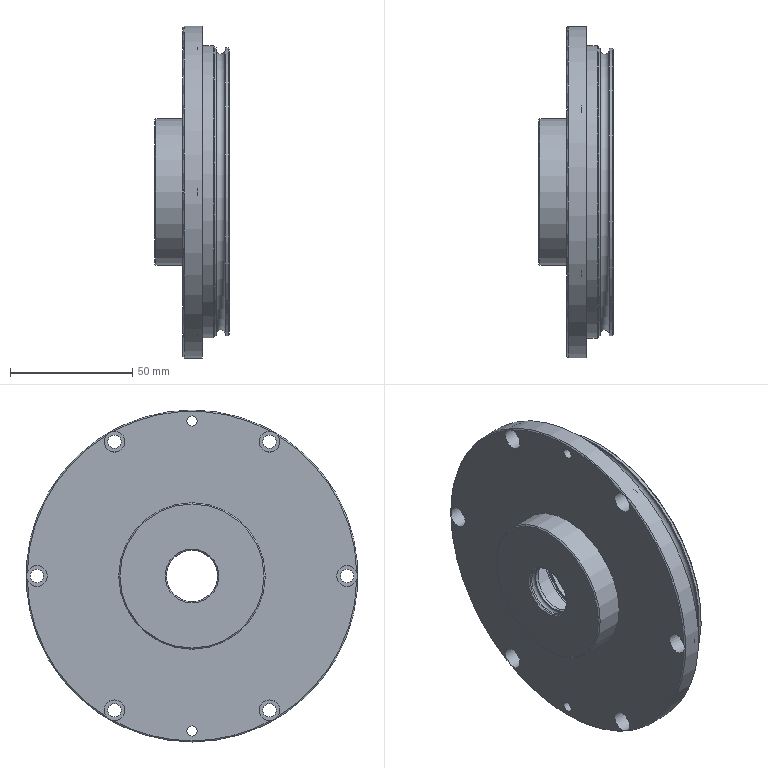Part | NX | features BREP 1 | 1 solid | 56 faces | box 30.5 x 136 x 136 mm | volume 150604 mm3 | cylinder 27 | plane 21 | cone 6 | torus 2 | commonest cylinder face diameters 5.5 x6 8.5 x6 4.2 x2 21 x2 47 x2 60 x2
STEP:
#1=CARTESIAN_POINT('',(13.3,0.,58.3));
#2=VERTEX_POINT('',#1);
#3=CARTESIAN_POINT('',(13.3,0.,0.));
#4=DIRECTION('',(-1.,0.,0.));
#5=DIRECTION('',(0.,0.,1.));
#6=AXIS2_PLACEMENT_3D('',#3,#4,#5);
#7=CIRCLE('',#6,58.3);
#8=EDGE_CURVE('',#2,#2,#7,.T.);
#9=ORIENTED_EDGE('',*,*,#8,.T.);
#10=EDGE_LOOP('',(#9));
#11=FACE_BOUND('',#10,.T.);
#12=CARTESIAN_POINT('',(9.7,0.,58.3));
#13=VERTEX_POINT('',#12);
#14=CARTESIAN_POINT('',(9.7,0.,0.));
#15=DIRECTION('',(-1.,0.,0.));
#16=DIRECTION('',(0.,0.,1.));
#17=AXIS2_PLACEMENT_3D('',#14,#15,#16);
#18=CIRCLE('',#17,58.3);
#19=EDGE_CURVE('',#13,#13,#18,.T.);
#20=ORIENTED_EDGE('',*,*,#19,.F.);
#21=EDGE_LOOP('',(#20));
#22=FACE_BOUND('',#21,.T.);
#23=CARTESIAN_POINT('',(11.5,0.,0.));
#24=DIRECTION('',(-1.,0.,0.));
#25=DIRECTION('',(0.,0.,1.));
#26=AXIS2_PLACEMENT_3D('',#23,#24,#25);
#27=TOROIDAL_SURFACE('',#26,58.3,1.8);
#28=ADVANCED_FACE('',(#11,#22),#27,.F.);
#29=CARTESIAN_POINT('',(8.5,0.,60.));
#30=VERTEX_POINT('',#29);
#31=CARTESIAN_POINT('',(8.5,0.,0.));
#32=DIRECTION('',(-1.,0.,0.));
#33=DIRECTION('',(0.,0.,1.));
#34=AXIS2_PLACEMENT_3D('',#31,#32,#33);
#35=CIRCLE('',#34,60.);
#36=EDGE_CURVE('',#30,#30,#35,.T.);
#37=ORIENTED_EDGE('',*,*,#36,.F.);
#38=EDGE_LOOP('',(#37));
#39=FACE_BOUND('',#38,.T.);
#40=CARTESIAN_POINT('',(9.,0.,59.5));
#41=VERTEX_POINT('',#40);
#42=CARTESIAN_POINT('',(9.,0.,0.));
#43=DIRECTION('',(1.,0.,0.));
#44=DIRECTION('',(0.,0.,1.));
#45=AXIS2_PLACEMENT_3D('',#42,#43,#44);
#46=CIRCLE('',#45,59.5);
#47=EDGE_CURVE('',#41,#41,#46,.T.);
#48=ORIENTED_EDGE('',*,*,#47,.F.);
#49=EDGE_LOOP('',(#48));
#50=FACE_BOUND('',#49,.T.);
#51=CARTESIAN_POINT('',(8.5,0.,0.));
#52=DIRECTION('',(-1.,0.,0.));
#53=DIRECTION('',(0.,0.,1.));
#54=AXIS2_PLACEMENT_3D('',#51,#52,#53);
#55=CONICAL_SURFACE('',#54,60.,0.7854);
#56=ADVANCED_FACE('',(#39,#50),#55,.T.);
#57=CARTESIAN_POINT('',(-4.,0.,65.6));
#58=VERTEX_POINT('',#57);
#59=CARTESIAN_POINT('',(-4.,0.,63.5));
#60=DIRECTION('',(-1.,0.,0.));
#61=DIRECTION('',(0.,0.,1.));
#62=AXIS2_PLACEMENT_3D('',#59,#60,#61);
#63=CIRCLE('',#62,2.1);
#64=EDGE_CURVE('',#58,#58,#63,.T.);
#65=ORIENTED_EDGE('',*,*,#64,.T.);
#66=EDGE_LOOP('',(#65));
#67=FACE_BOUND('',#66,.T.);
#68=CARTESIAN_POINT('',(4.,0.,65.6));
#69=VERTEX_POINT('',#68);
#70=CARTESIAN_POINT('',(4.,0.,63.5));
#71=DIRECTION('',(-1.,0.,0.));
#72=DIRECTION('',(0.,0.,1.));
#73=AXIS2_PLACEMENT_3D('',#70,#71,#72);
#74=CIRCLE('',#73,2.1);
#75=EDGE_CURVE('',#69,#69,#74,.T.);
#76=ORIENTED_EDGE('',*,*,#75,.F.);
#77=EDGE_LOOP('',(#76));
#78=FACE_BOUND('',#77,.T.);
#79=CARTESIAN_POINT('',(-4.,0.,63.5));
#80=DIRECTION('',(-1.,0.,0.));
#81=DIRECTION('',(0.,0.,1.));
#82=AXIS2_PLACEMENT_3D('',#79,#80,#81);
#83=CYLINDRICAL_SURFACE('',#82,2.1);
#84=ADVANCED_FACE('',(#67,#78),#83,.F.);
#85=CARTESIAN_POINT('',(-4.,0.,-61.4));
#86=VERTEX_POINT('',#85);
#87=CARTESIAN_POINT('',(-4.,0.,-63.5));
#88=DIRECTION('',(-1.,0.,0.));
#89=DIRECTION('',(0.,0.,1.));
#90=AXIS2_PLACEMENT_3D('',#87,#88,#89);
#91=CIRCLE('',#90,2.1);
#92=EDGE_CURVE('',#86,#86,#91,.T.);
#93=ORIENTED_EDGE('',*,*,#92,.T.);
#94=EDGE_LOOP('',(#93));
#95=FACE_BOUND('',#94,.T.);
#96=CARTESIAN_POINT('',(4.,0.,-61.4));
#97=VERTEX_POINT('',#96);
#98=CARTESIAN_POINT('',(4.,0.,-63.5));
#99=DIRECTION('',(-1.,0.,0.));
#100=DIRECTION('',(0.,0.,1.));
#101=AXIS2_PLACEMENT_3D('',#98,#99,#100);
#102=CIRCLE('',#101,2.1);
#103=EDGE_CURVE('',#97,#97,#102,.T.);
#104=ORIENTED_EDGE('',*,*,#103,.F.);
#105=EDGE_LOOP('',(#104));
#106=FACE_BOUND('',#105,.T.);
#107=CARTESIAN_POINT('',(-4.,0.,-63.5));
#108=DIRECTION('',(-1.,0.,0.));
#109=DIRECTION('',(0.,0.,1.));
#110=AXIS2_PLACEMENT_3D('',#107,#108,#109);
#111=CYLINDRICAL_SURFACE('',#110,2.1);
#112=ADVANCED_FACE('',(#95,#106),#111,.F.);
#113=CARTESIAN_POINT('',(-4.,35.024,57.702));
#114=VERTEX_POINT('',#113);
#115=CARTESIAN_POINT('',(-4.,32.46,59.183));
#116=VERTEX_POINT('',#115);
#117=CARTESIAN_POINT('',(-4.,31.75,54.993));
#118=DIRECTION('',(-1.,0.,0.));
#119=DIRECTION('',(0.,0.,1.));
#120=AXIS2_PLACEMENT_3D('',#117,#118,#119);
#121=CIRCLE('',#120,4.25);
#122=EDGE_CURVE('',#114,#116,#121,.T.);
#123=ORIENTED_EDGE('',*,*,#122,.T.);
#124=CARTESIAN_POINT('',(-4.,32.46,59.183));
#125=CARTESIAN_POINT('',(-3.678,33.429,59.019));
#126=CARTESIAN_POINT('',(-3.678,34.397,58.46));
#127=CARTESIAN_POINT('',(-4.,35.024,57.702));
#128=B_SPLINE_CURVE_WITH_KNOTS('',3,(#124,#125,#126,#127),.UNSPECIFIED.,.F.,.F.,(4,4),(0.,0.003063),.UNSPECIFIED.);
#129=EDGE_CURVE('',#116,#114,#128,.T.);
#130=ORIENTED_EDGE('',*,*,#129,.T.);
#131=EDGE_LOOP('',(#123,#130));
#132=FACE_BOUND('',#131,.T.);
#133=CARTESIAN_POINT('',(1.8,31.75,59.243));
#134=VERTEX_POINT('',#133);
#135=CARTESIAN_POINT('',(1.8,31.75,54.993));
#136=DIRECTION('',(-1.,0.,0.));
#137=DIRECTION('',(0.,0.,1.));
#138=AXIS2_PLACEMENT_3D('',#135,#136,#137);
#139=CIRCLE('',#138,4.25);
#140=EDGE_CURVE('',#134,#134,#139,.T.);
#141=ORIENTED_EDGE('',*,*,#140,.F.);
#142=EDGE_LOOP('',(#141));
#143=FACE_BOUND('',#142,.T.);
#144=CARTESIAN_POINT('',(-4.,31.75,54.993));
#145=DIRECTION('',(-1.,0.,0.));
#146=DIRECTION('',(0.,0.,1.));
#147=AXIS2_PLACEMENT_3D('',#144,#145,#146);
#148=CYLINDRICAL_SURFACE('',#147,4.25);
#149=ADVANCED_FACE('',(#132,#143),#148,.F.);
#150=CARTESIAN_POINT('',(1.8,31.75,57.743));
#151=VERTEX_POINT('',#150);
#152=CARTESIAN_POINT('',(1.8,31.75,54.993));
#153=DIRECTION('',(-1.,0.,0.));
#154=DIRECTION('',(0.,0.,1.));
#155=AXIS2_PLACEMENT_3D('',#152,#153,#154);
#156=CIRCLE('',#155,2.75);
#157=EDGE_CURVE('',#151,#151,#156,.T.);
#158=ORIENTED_EDGE('',*,*,#157,.T.);
#159=EDGE_LOOP('',(#158));
#160=FACE_BOUND('',#159,.T.);
#161=CARTESIAN_POINT('',(4.,31.75,57.743));
#162=VERTEX_POINT('',#161);
#163=CARTESIAN_POINT('',(4.,31.75,54.993));
#164=DIRECTION('',(-1.,0.,0.));
#165=DIRECTION('',(0.,0.,1.));
#166=AXIS2_PLACEMENT_3D('',#163,#164,#165);
#167=CIRCLE('',#166,2.75);
#168=EDGE_CURVE('',#162,#162,#167,.T.);
#169=ORIENTED_EDGE('',*,*,#168,.F.);
#170=EDGE_LOOP('',(#169));
#171=FACE_BOUND('',#170,.T.);
#172=CARTESIAN_POINT('',(-4.,31.75,54.993));
#173=DIRECTION('',(-1.,0.,0.));
#174=DIRECTION('',(0.,0.,1.));
#175=AXIS2_PLACEMENT_3D('',#172,#173,#174);
#176=CYLINDRICAL_SURFACE('',#175,2.75);
#177=ADVANCED_FACE('',(#160,#171),#176,.F.);
#178=CARTESIAN_POINT('',(-4.,-35.024,57.702));
#179=VERTEX_POINT('',#178);
#180=CARTESIAN_POINT('',(-4.,-32.46,59.183));
#181=VERTEX_POINT('',#180);
#182=CARTESIAN_POINT('',(-4.,-35.024,57.702));
#183=CARTESIAN_POINT('',(-3.678,-34.398,58.459));
#184=CARTESIAN_POINT('',(-3.678,-33.429,59.019));
#185=CARTESIAN_POINT('',(-4.,-32.46,59.183));
#186=B_SPLINE_CURVE_WITH_KNOTS('',3,(#182,#183,#184,#185),.UNSPECIFIED.,.F.,.F.,(4,4),(0.,0.003063),.UNSPECIFIED.);
#187=EDGE_CURVE('',#179,#181,#186,.T.);
#188=ORIENTED_EDGE('',*,*,#187,.T.);
#189=CARTESIAN_POINT('',(-4.,-31.75,54.993));
#190=DIRECTION('',(-1.,0.,0.));
#191=DIRECTION('',(0.,0.,1.));
#192=AXIS2_PLACEMENT_3D('',#189,#190,#191);
#193=CIRCLE('',#192,4.25);
#194=EDGE_CURVE('',#181,#179,#193,.T.);
#195=ORIENTED_EDGE('',*,*,#194,.T.);
#196=EDGE_LOOP('',(#188,#195));
#197=FACE_BOUND('',#196,.T.);
#198=CARTESIAN_POINT('',(1.8,-31.75,59.243));
#199=VERTEX_POINT('',#198);
#200=CARTESIAN_POINT('',(1.8,-31.75,54.993));
#201=DIRECTION('',(-1.,0.,0.));
#202=DIRECTION('',(0.,0.,1.));
#203=AXIS2_PLACEMENT_3D('',#200,#201,#202);
#204=CIRCLE('',#203,4.25);
#205=EDGE_CURVE('',#199,#199,#204,.T.);
#206=ORIENTED_EDGE('',*,*,#205,.F.);
#207=EDGE_LOOP('',(#206));
#208=FACE_BOUND('',#207,.T.);
#209=CARTESIAN_POINT('',(-4.,-31.75,54.993));
#210=DIRECTION('',(-1.,0.,0.));
#211=DIRECTION('',(0.,0.,1.));
#212=AXIS2_PLACEMENT_3D('',#209,#210,#211);
#213=CYLINDRICAL_SURFACE('',#212,4.25);
#214=ADVANCED_FACE('',(#197,#208),#213,.F.);
#215=CARTESIAN_POINT('',(1.8,-31.75,57.743));
#216=VERTEX_POINT('',#215);
#217=CARTESIAN_POINT('',(1.8,-31.75,54.993));
#218=DIRECTION('',(-1.,0.,0.));
#219=DIRECTION('',(0.,0.,1.));
#220=AXIS2_PLACEMENT_3D('',#217,#218,#219);
#221=CIRCLE('',#220,2.75);
#222=EDGE_CURVE('',#216,#216,#221,.T.);
#223=ORIENTED_EDGE('',*,*,#222,.T.);
#224=EDGE_LOOP('',(#223));
#225=FACE_BOUND('',#224,.T.);
#226=CARTESIAN_POINT('',(4.,-31.75,57.743));
#227=VERTEX_POINT('',#226);
#228=CARTESIAN_POINT('',(4.,-31.75,54.993));
#229=DIRECTION('',(-1.,0.,0.));
#230=DIRECTION('',(0.,0.,1.));
#231=AXIS2_PLACEMENT_3D('',#228,#229,#230);
#232=CIRCLE('',#231,2.75);
#233=EDGE_CURVE('',#227,#227,#232,.T.);
#234=ORIENTED_EDGE('',*,*,#233,.F.);
#235=EDGE_LOOP('',(#234));
#236=FACE_BOUND('',#235,.T.);
#237=CARTESIAN_POINT('',(-4.,-31.75,54.993));
#238=DIRECTION('',(-1.,0.,0.));
#239=DIRECTION('',(0.,0.,1.));
#240=AXIS2_PLACEMENT_3D('',#237,#238,#239);
#241=CYLINDRICAL_SURFACE('',#240,2.75);
#242=ADVANCED_FACE('',(#225,#236),#241,.F.);
#243=CARTESIAN_POINT('',(-4.,-67.484,-1.481));
#244=VERTEX_POINT('',#243);
#245=CARTESIAN_POINT('',(-4.,-67.484,1.481));
#246=VERTEX_POINT('',#245);
#247=CARTESIAN_POINT('',(-4.,-67.484,-1.481));
#248=CARTESIAN_POINT('',(-3.678,-67.826,-0.5594));
#249=CARTESIAN_POINT('',(-3.678,-67.826,0.5591));
#250=CARTESIAN_POINT('',(-4.,-67.484,1.481));
#251=B_SPLINE_CURVE_WITH_KNOTS('',3,(#247,#248,#249,#250),.UNSPECIFIED.,.F.,.F.,(4,4),(0.,0.003063),.UNSPECIFIED.);
#252=EDGE_CURVE('',#244,#246,#251,.T.);
#253=ORIENTED_EDGE('',*,*,#252,.T.);
#254=CARTESIAN_POINT('',(-4.,-63.5,0.));
#255=DIRECTION('',(-1.,0.,0.));
#256=DIRECTION('',(0.,0.,1.));
#257=AXIS2_PLACEMENT_3D('',#254,#255,#256);
#258=CIRCLE('',#257,4.25);
#259=EDGE_CURVE('',#246,#244,#258,.T.);
#260=ORIENTED_EDGE('',*,*,#259,.T.);
#261=EDGE_LOOP('',(#253,#260));
#262=FACE_BOUND('',#261,.T.);
#263=CARTESIAN_POINT('',(1.8,-63.5,4.25));
#264=VERTEX_POINT('',#263);
#265=CARTESIAN_POINT('',(1.8,-63.5,0.));
#266=DIRECTION('',(-1.,0.,0.));
#267=DIRECTION('',(0.,0.,1.));
#268=AXIS2_PLACEMENT_3D('',#265,#266,#267);
#269=CIRCLE('',#268,4.25);
#270=EDGE_CURVE('',#264,#264,#269,.T.);
#271=ORIENTED_EDGE('',*,*,#270,.F.);
#272=EDGE_LOOP('',(#271));
#273=FACE_BOUND('',#272,.T.);
#274=CARTESIAN_POINT('',(-4.,-63.5,0.));
#275=DIRECTION('',(-1.,0.,0.));
#276=DIRECTION('',(0.,0.,1.));
#277=AXIS2_PLACEMENT_3D('',#274,#275,#276);
#278=CYLINDRICAL_SURFACE('',#277,4.25);
#279=ADVANCED_FACE('',(#262,#273),#278,.F.);
#280=CARTESIAN_POINT('',(1.8,-63.5,2.75));
#281=VERTEX_POINT('',#280);
#282=CARTESIAN_POINT('',(1.8,-63.5,0.));
#283=DIRECTION('',(-1.,0.,0.));
#284=DIRECTION('',(0.,0.,1.));
#285=AXIS2_PLACEMENT_3D('',#282,#283,#284);
#286=CIRCLE('',#285,2.75);
#287=EDGE_CURVE('',#281,#281,#286,.T.);
#288=ORIENTED_EDGE('',*,*,#287,.T.);
#289=EDGE_LOOP('',(#288));
#290=FACE_BOUND('',#289,.T.);
#291=CARTESIAN_POINT('',(4.,-63.5,2.75));
#292=VERTEX_POINT('',#291);
#293=CARTESIAN_POINT('',(4.,-63.5,0.));
#294=DIRECTION('',(-1.,0.,0.));
#295=DIRECTION('',(0.,0.,1.));
#296=AXIS2_PLACEMENT_3D('',#293,#294,#295);
#297=CIRCLE('',#296,2.75);
#298=EDGE_CURVE('',#292,#292,#297,.T.);
#299=ORIENTED_EDGE('',*,*,#298,.F.);
#300=EDGE_LOOP('',(#299));
#301=FACE_BOUND('',#300,.T.);
#302=CARTESIAN_POINT('',(-4.,-63.5,0.));
#303=DIRECTION('',(-1.,0.,0.));
#304=DIRECTION('',(0.,0.,1.));
#305=AXIS2_PLACEMENT_3D('',#302,#303,#304);
#306=CYLINDRICAL_SURFACE('',#305,2.75);
#307=ADVANCED_FACE('',(#290,#301),#306,.F.);
#308=CARTESIAN_POINT('',(-4.,-32.46,-59.183));
#309=VERTEX_POINT('',#308);
#310=CARTESIAN_POINT('',(-4.,-35.024,-57.702));
#311=VERTEX_POINT('',#310);
#312=CARTESIAN_POINT('',(-4.,-32.46,-59.183));
#313=CARTESIAN_POINT('',(-3.678,-33.429,-59.019));
#314=CARTESIAN_POINT('',(-3.678,-34.397,-58.46));
#315=CARTESIAN_POINT('',(-4.,-35.024,-57.702));
#316=B_SPLINE_CURVE_WITH_KNOTS('',3,(#312,#313,#314,#315),.UNSPECIFIED.,.F.,.F.,(4,4),(0.,0.003063),.UNSPECIFIED.);
#317=EDGE_CURVE('',#309,#311,#316,.T.);
#318=ORIENTED_EDGE('',*,*,#317,.T.);
#319=CARTESIAN_POINT('',(-4.,-31.75,-54.993));
#320=DIRECTION('',(-1.,0.,0.));
#321=DIRECTION('',(0.,0.,1.));
#322=AXIS2_PLACEMENT_3D('',#319,#320,#321);
#323=CIRCLE('',#322,4.25);
#324=EDGE_CURVE('',#311,#309,#323,.T.);
#325=ORIENTED_EDGE('',*,*,#324,.T.);
#326=EDGE_LOOP('',(#318,#325));
#327=FACE_BOUND('',#326,.T.);
#328=CARTESIAN_POINT('',(1.8,-31.75,-50.743));
#329=VERTEX_POINT('',#328);
#330=CARTESIAN_POINT('',(1.8,-31.75,-54.993));
#331=DIRECTION('',(-1.,0.,0.));
#332=DIRECTION('',(0.,0.,1.));
#333=AXIS2_PLACEMENT_3D('',#330,#331,#332);
#334=CIRCLE('',#333,4.25);
#335=EDGE_CURVE('',#329,#329,#334,.T.);
#336=ORIENTED_EDGE('',*,*,#335,.F.);
#337=EDGE_LOOP('',(#336));
#338=FACE_BOUND('',#337,.T.);
#339=CARTESIAN_POINT('',(-4.,-31.75,-54.993));
#340=DIRECTION('',(-1.,0.,0.));
#341=DIRECTION('',(0.,0.,1.));
#342=AXIS2_PLACEMENT_3D('',#339,#340,#341);
#343=CYLINDRICAL_SURFACE('',#342,4.25);
#344=ADVANCED_FACE('',(#327,#338),#343,.F.);
#345=CARTESIAN_POINT('',(1.8,-31.75,-52.243));
#346=VERTEX_POINT('',#345);
#347=CARTESIAN_POINT('',(1.8,-31.75,-54.993));
#348=DIRECTION('',(-1.,0.,0.));
#349=DIRECTION('',(0.,0.,1.));
#350=AXIS2_PLACEMENT_3D('',#347,#348,#349);
#351=CIRCLE('',#350,2.75);
#352=EDGE_CURVE('',#346,#346,#351,.T.);
#353=ORIENTED_EDGE('',*,*,#352,.T.);
#354=EDGE_LOOP('',(#353));
#355=FACE_BOUND('',#354,.T.);
#356=CARTESIAN_POINT('',(4.,-31.75,-52.243));
#357=VERTEX_POINT('',#356);
#358=CARTESIAN_POINT('',(4.,-31.75,-54.993));
#359=DIRECTION('',(-1.,0.,0.));
#360=DIRECTION('',(0.,0.,1.));
#361=AXIS2_PLACEMENT_3D('',#358,#359,#360);
#362=CIRCLE('',#361,2.75);
#363=EDGE_CURVE('',#357,#357,#362,.T.);
#364=ORIENTED_EDGE('',*,*,#363,.F.);
#365=EDGE_LOOP('',(#364));
#366=FACE_BOUND('',#365,.T.);
#367=CARTESIAN_POINT('',(-4.,-31.75,-54.993));
#368=DIRECTION('',(-1.,0.,0.));
#369=DIRECTION('',(0.,0.,1.));
#370=AXIS2_PLACEMENT_3D('',#367,#368,#369);
#371=CYLINDRICAL_SURFACE('',#370,2.75);
#372=ADVANCED_FACE('',(#355,#366),#371,.F.);
#373=CARTESIAN_POINT('',(-4.,32.46,-59.183));
#374=VERTEX_POINT('',#373);
#375=CARTESIAN_POINT('',(-4.,35.024,-57.702));
#376=VERTEX_POINT('',#375);
#377=CARTESIAN_POINT('',(-4.,31.75,-54.993));
#378=DIRECTION('',(-1.,0.,0.));
#379=DIRECTION('',(0.,0.,1.));
#380=AXIS2_PLACEMENT_3D('',#377,#378,#379);
#381=CIRCLE('',#380,4.25);
#382=EDGE_CURVE('',#374,#376,#381,.T.);
#383=ORIENTED_EDGE('',*,*,#382,.T.);
#384=CARTESIAN_POINT('',(-4.,35.024,-57.702));
#385=CARTESIAN_POINT('',(-3.678,34.398,-58.459));
#386=CARTESIAN_POINT('',(-3.678,33.429,-59.019));
#387=CARTESIAN_POINT('',(-4.,32.46,-59.183));
#388=B_SPLINE_CURVE_WITH_KNOTS('',3,(#384,#385,#386,#387),.UNSPECIFIED.,.F.,.F.,(4,4),(0.,0.003063),.UNSPECIFIED.);
#389=EDGE_CURVE('',#376,#374,#388,.T.);
#390=ORIENTED_EDGE('',*,*,#389,.T.);
#391=EDGE_LOOP('',(#383,#390));
#392=FACE_BOUND('',#391,.T.);
#393=CARTESIAN_POINT('',(1.8,31.75,-50.743));
#394=VERTEX_POINT('',#393);
#395=CARTESIAN_POINT('',(1.8,31.75,-54.993));
#396=DIRECTION('',(-1.,0.,0.));
#397=DIRECTION('',(0.,0.,1.));
#398=AXIS2_PLACEMENT_3D('',#395,#396,#397);
#399=CIRCLE('',#398,4.25);
#400=EDGE_CURVE('',#394,#394,#399,.T.);
#401=ORIENTED_EDGE('',*,*,#400,.F.);
#402=EDGE_LOOP('',(#401));
#403=FACE_BOUND('',#402,.T.);
#404=CARTESIAN_POINT('',(-4.,31.75,-54.993));
#405=DIRECTION('',(-1.,0.,0.));
#406=DIRECTION('',(0.,0.,1.));
#407=AXIS2_PLACEMENT_3D('',#404,#405,#406);
#408=CYLINDRICAL_SURFACE('',#407,4.25);
#409=ADVANCED_FACE('',(#392,#403),#408,.F.);
#410=CARTESIAN_POINT('',(1.8,31.75,-52.243));
#411=VERTEX_POINT('',#410);
#412=CARTESIAN_POINT('',(1.8,31.75,-54.993));
#413=DIRECTION('',(-1.,0.,0.));
#414=DIRECTION('',(0.,0.,1.));
#415=AXIS2_PLACEMENT_3D('',#412,#413,#414);
#416=CIRCLE('',#415,2.75);
#417=EDGE_CURVE('',#411,#411,#416,.T.);
#418=ORIENTED_EDGE('',*,*,#417,.T.);
#419=EDGE_LOOP('',(#418));
#420=FACE_BOUND('',#419,.T.);
#421=CARTESIAN_POINT('',(4.,31.75,-52.243));
#422=VERTEX_POINT('',#421);
#423=CARTESIAN_POINT('',(4.,31.75,-54.993));
#424=DIRECTION('',(-1.,0.,0.));
#425=DIRECTION('',(0.,0.,1.));
#426=AXIS2_PLACEMENT_3D('',#423,#424,#425);
#427=CIRCLE('',#426,2.75);
#428=EDGE_CURVE('',#422,#422,#427,.T.);
#429=ORIENTED_EDGE('',*,*,#428,.F.);
#430=EDGE_LOOP('',(#429));
#431=FACE_BOUND('',#430,.T.);
#432=CARTESIAN_POINT('',(-4.,31.75,-54.993));
#433=DIRECTION('',(-1.,0.,0.));
#434=DIRECTION('',(0.,0.,1.));
#435=AXIS2_PLACEMENT_3D('',#432,#433,#434);
#436=CYLINDRICAL_SURFACE('',#435,2.75);
#437=ADVANCED_FACE('',(#420,#431),#436,.F.);
#438=CARTESIAN_POINT('',(-4.,67.484,-1.481));
#439=VERTEX_POINT('',#438);
#440=CARTESIAN_POINT('',(-4.,67.484,1.481));
#441=VERTEX_POINT('',#440);
#442=CARTESIAN_POINT('',(-4.,63.5,0.));
#443=DIRECTION('',(-1.,0.,0.));
#444=DIRECTION('',(0.,0.,1.));
#445=AXIS2_PLACEMENT_3D('',#442,#443,#444);
#446=CIRCLE('',#445,4.25);
#447=EDGE_CURVE('',#439,#441,#446,.T.);
#448=ORIENTED_EDGE('',*,*,#447,.T.);
#449=CARTESIAN_POINT('',(-4.,67.484,1.481));
#450=CARTESIAN_POINT('',(-3.678,67.826,0.5594));
#451=CARTESIAN_POINT('',(-3.678,67.826,-0.5591));
#452=CARTESIAN_POINT('',(-4.,67.484,-1.481));
#453=B_SPLINE_CURVE_WITH_KNOTS('',3,(#449,#450,#451,#452),.UNSPECIFIED.,.F.,.F.,(4,4),(0.,0.003063),.UNSPECIFIED.);
#454=EDGE_CURVE('',#441,#439,#453,.T.);
#455=ORIENTED_EDGE('',*,*,#454,.T.);
#456=EDGE_LOOP('',(#448,#455));
#457=FACE_BOUND('',#456,.T.);
#458=CARTESIAN_POINT('',(1.8,63.5,4.25));
#459=VERTEX_POINT('',#458);
#460=CARTESIAN_POINT('',(1.8,63.5,0.));
#461=DIRECTION('',(-1.,0.,0.));
#462=DIRECTION('',(0.,0.,1.));
#463=AXIS2_PLACEMENT_3D('',#460,#461,#462);
#464=CIRCLE('',#463,4.25);
#465=EDGE_CURVE('',#459,#459,#464,.T.);
#466=ORIENTED_EDGE('',*,*,#465,.F.);
#467=EDGE_LOOP('',(#466));
#468=FACE_BOUND('',#467,.T.);
#469=CARTESIAN_POINT('',(-4.,63.5,0.));
#470=DIRECTION('',(-1.,0.,0.));
#471=DIRECTION('',(0.,0.,1.));
#472=AXIS2_PLACEMENT_3D('',#469,#470,#471);
#473=CYLINDRICAL_SURFACE('',#472,4.25);
#474=ADVANCED_FACE('',(#457,#468),#473,.F.);
#475=CARTESIAN_POINT('',(1.8,63.5,2.75));
#476=VERTEX_POINT('',#475);
#477=CARTESIAN_POINT('',(1.8,63.5,0.));
#478=DIRECTION('',(-1.,0.,0.));
#479=DIRECTION('',(0.,0.,1.));
#480=AXIS2_PLACEMENT_3D('',#477,#478,#479);
#481=CIRCLE('',#480,2.75);
#482=EDGE_CURVE('',#476,#476,#481,.T.);
#483=ORIENTED_EDGE('',*,*,#482,.T.);
#484=EDGE_LOOP('',(#483));
#485=FACE_BOUND('',#484,.T.);
#486=CARTESIAN_POINT('',(4.,63.5,2.75));
#487=VERTEX_POINT('',#486);
#488=CARTESIAN_POINT('',(4.,63.5,0.));
#489=DIRECTION('',(-1.,0.,0.));
#490=DIRECTION('',(0.,0.,1.));
#491=AXIS2_PLACEMENT_3D('',#488,#489,#490);
#492=CIRCLE('',#491,2.75);
#493=EDGE_CURVE('',#487,#487,#492,.T.);
#494=ORIENTED_EDGE('',*,*,#493,.F.);
#495=EDGE_LOOP('',(#494));
#496=FACE_BOUND('',#495,.T.);
#497=CARTESIAN_POINT('',(-4.,63.5,0.));
#498=DIRECTION('',(-1.,0.,0.));
#499=DIRECTION('',(0.,0.,1.));
#500=AXIS2_PLACEMENT_3D('',#497,#498,#499);
#501=CYLINDRICAL_SURFACE('',#500,2.75);
#502=ADVANCED_FACE('',(#485,#496),#501,.F.);
#503=CARTESIAN_POINT('',(-3.5,0.,-68.));
#504=VERTEX_POINT('',#503);
#505=CARTESIAN_POINT('',(-3.5,0.,0.));
#506=DIRECTION('',(1.,0.,0.));
#507=DIRECTION('',(0.,0.,-1.));
#508=AXIS2_PLACEMENT_3D('',#505,#506,#507);
#509=CIRCLE('',#508,68.);
#510=EDGE_CURVE('',#504,#504,#509,.T.);
#511=ORIENTED_EDGE('',*,*,#510,.F.);
#512=EDGE_LOOP('',(#511));
#513=FACE_BOUND('',#512,.T.);
#514=CARTESIAN_POINT('',(-4.,0.,0.));
#515=DIRECTION('',(-1.,0.,0.));
#516=DIRECTION('',(0.,0.,-1.));
#517=AXIS2_PLACEMENT_3D('',#514,#515,#516);
#518=CIRCLE('',#517,67.5);
#519=EDGE_CURVE('',#181,#116,#518,.T.);
#520=ORIENTED_EDGE('',*,*,#519,.F.);
#521=ORIENTED_EDGE('',*,*,#187,.F.);
#522=CARTESIAN_POINT('',(-4.,0.,0.));
#523=DIRECTION('',(-1.,0.,0.));
#524=DIRECTION('',(0.,0.,-1.));
#525=AXIS2_PLACEMENT_3D('',#522,#523,#524);
#526=CIRCLE('',#525,67.5);
#527=EDGE_CURVE('',#246,#179,#526,.T.);
#528=ORIENTED_EDGE('',*,*,#527,.F.);
#529=ORIENTED_EDGE('',*,*,#252,.F.);
#530=CARTESIAN_POINT('',(-4.,0.,0.));
#531=DIRECTION('',(-1.,0.,0.));
#532=DIRECTION('',(0.,0.,-1.));
#533=AXIS2_PLACEMENT_3D('',#530,#531,#532);
#534=CIRCLE('',#533,67.5);
#535=EDGE_CURVE('',#311,#244,#534,.T.);
#536=ORIENTED_EDGE('',*,*,#535,.F.);
#537=ORIENTED_EDGE('',*,*,#317,.F.);
#538=CARTESIAN_POINT('',(-4.,0.,0.));
#539=DIRECTION('',(-1.,0.,0.));
#540=DIRECTION('',(0.,0.,-1.));
#541=AXIS2_PLACEMENT_3D('',#538,#539,#540);
#542=CIRCLE('',#541,67.5);
#543=EDGE_CURVE('',#374,#309,#542,.T.);
#544=ORIENTED_EDGE('',*,*,#543,.F.);
#545=ORIENTED_EDGE('',*,*,#389,.F.);
#546=CARTESIAN_POINT('',(-4.,0.,0.));
#547=DIRECTION('',(-1.,0.,0.));
#548=DIRECTION('',(0.,0.,-1.));
#549=AXIS2_PLACEMENT_3D('',#546,#547,#548);
#550=CIRCLE('',#549,67.5);
#551=EDGE_CURVE('',#439,#376,#550,.T.);
#552=ORIENTED_EDGE('',*,*,#551,.F.);
#553=ORIENTED_EDGE('',*,*,#454,.F.);
#554=CARTESIAN_POINT('',(-4.,0.,0.));
#555=DIRECTION('',(-1.,0.,0.));
#556=DIRECTION('',(0.,0.,-1.));
#557=AXIS2_PLACEMENT_3D('',#554,#555,#556);
#558=CIRCLE('',#557,67.5);
#559=EDGE_CURVE('',#114,#441,#558,.T.);
#560=ORIENTED_EDGE('',*,*,#559,.F.);
#561=ORIENTED_EDGE('',*,*,#129,.F.);
#562=EDGE_LOOP('',(#520,#521,#528,#529,#536,#537,#544,#545,#552,#553,#560,#561));
#563=FACE_BOUND('',#562,.T.);
#564=CARTESIAN_POINT('',(-4.,0.,0.));
#565=DIRECTION('',(1.,0.,0.));
#566=DIRECTION('',(0.,0.,-1.));
#567=AXIS2_PLACEMENT_3D('',#564,#565,#566);
#568=CONICAL_SURFACE('',#567,67.5,0.7854);
#569=ADVANCED_FACE('',(#513,#563),#568,.T.);
#570=CARTESIAN_POINT('',(-15.,0.,-30.));
#571=VERTEX_POINT('',#570);
#572=CARTESIAN_POINT('',(-15.,0.,0.));
#573=DIRECTION('',(1.,0.,0.));
#574=DIRECTION('',(0.,0.,-1.));
#575=AXIS2_PLACEMENT_3D('',#572,#573,#574);
#576=CIRCLE('',#575,30.);
#577=EDGE_CURVE('',#571,#571,#576,.T.);
#578=ORIENTED_EDGE('',*,*,#577,.F.);
#579=EDGE_LOOP('',(#578));
#580=FACE_BOUND('',#579,.T.);
#581=CARTESIAN_POINT('',(-15.5,0.,-29.5));
#582=VERTEX_POINT('',#581);
#583=CARTESIAN_POINT('',(-15.5,0.,0.));
#584=DIRECTION('',(-1.,0.,0.));
#585=DIRECTION('',(0.,0.,-1.));
#586=AXIS2_PLACEMENT_3D('',#583,#584,#585);
#587=CIRCLE('',#586,29.5);
#588=EDGE_CURVE('',#582,#582,#587,.T.);
#589=ORIENTED_EDGE('',*,*,#588,.F.);
#590=EDGE_LOOP('',(#589));
#591=FACE_BOUND('',#590,.T.);
#592=CARTESIAN_POINT('',(-15.5,0.,0.));
#593=DIRECTION('',(1.,0.,0.));
#594=DIRECTION('',(0.,0.,-1.));
#595=AXIS2_PLACEMENT_3D('',#592,#593,#594);
#596=CONICAL_SURFACE('',#595,29.5,0.7854);
#597=ADVANCED_FACE('',(#580,#591),#596,.T.);
#598=CARTESIAN_POINT('',(-15.5,0.,-11.));
#599=VERTEX_POINT('',#598);
#600=CARTESIAN_POINT('',(-15.5,0.,0.));
#601=DIRECTION('',(1.,0.,0.));
#602=DIRECTION('',(0.,0.,-1.));
#603=AXIS2_PLACEMENT_3D('',#600,#601,#602);
#604=CIRCLE('',#603,11.);
#605=EDGE_CURVE('',#599,#599,#604,.T.);
#606=ORIENTED_EDGE('',*,*,#605,.F.);
#607=EDGE_LOOP('',(#606));
#608=FACE_BOUND('',#607,.T.);
#609=CARTESIAN_POINT('',(-15.,0.,-10.5));
#610=VERTEX_POINT('',#609);
#611=CARTESIAN_POINT('',(-15.,0.,0.));
#612=DIRECTION('',(-1.,0.,0.));
#613=DIRECTION('',(0.,0.,-1.));
#614=AXIS2_PLACEMENT_3D('',#611,#612,#613);
#615=CIRCLE('',#614,10.5);
#616=EDGE_CURVE('',#610,#610,#615,.T.);
#617=ORIENTED_EDGE('',*,*,#616,.F.);
#618=EDGE_LOOP('',(#617));
#619=FACE_BOUND('',#618,.T.);
#620=CARTESIAN_POINT('',(-15.,0.,0.));
#621=DIRECTION('',(-1.,0.,0.));
#622=DIRECTION('',(0.,0.,1.));
#623=AXIS2_PLACEMENT_3D('',#620,#621,#622);
#624=CONICAL_SURFACE('',#623,10.5,0.7854);
#625=ADVANCED_FACE('',(#608,#619),#624,.F.);
#626=CARTESIAN_POINT('',(9.,0.,24.));
#627=VERTEX_POINT('',#626);
#628=CARTESIAN_POINT('',(9.,0.,0.));
#629=DIRECTION('',(-1.,0.,0.));
#630=DIRECTION('',(0.,0.,1.));
#631=AXIS2_PLACEMENT_3D('',#628,#629,#630);
#632=CIRCLE('',#631,24.);
#633=EDGE_CURVE('',#627,#627,#632,.T.);
#634=ORIENTED_EDGE('',*,*,#633,.F.);
#635=EDGE_LOOP('',(#634));
#636=FACE_BOUND('',#635,.T.);
#637=CARTESIAN_POINT('',(8.5,0.,23.5));
#638=VERTEX_POINT('',#637);
#639=CARTESIAN_POINT('',(8.5,0.,0.));
#640=DIRECTION('',(1.,0.,0.));
#641=DIRECTION('',(0.,0.,1.));
#642=AXIS2_PLACEMENT_3D('',#639,#640,#641);
#643=CIRCLE('',#642,23.5);
#644=EDGE_CURVE('',#638,#638,#643,.T.);
#645=ORIENTED_EDGE('',*,*,#644,.F.);
#646=EDGE_LOOP('',(#645));
#647=FACE_BOUND('',#646,.T.);
#648=CARTESIAN_POINT('',(9.,0.,0.));
#649=DIRECTION('',(1.,0.,0.));
#650=DIRECTION('',(0.,0.,-1.));
#651=AXIS2_PLACEMENT_3D('',#648,#649,#650);
#652=CONICAL_SURFACE('',#651,24.,0.7854);
#653=ADVANCED_FACE('',(#636,#647),#652,.F.);
#654=CARTESIAN_POINT('',(14.5,0.,59.));
#655=VERTEX_POINT('',#654);
#656=CARTESIAN_POINT('',(14.5,0.,0.));
#657=DIRECTION('',(-1.,0.,0.));
#658=DIRECTION('',(0.,0.,1.));
#659=AXIS2_PLACEMENT_3D('',#656,#657,#658);
#660=CIRCLE('',#659,59.);
#661=EDGE_CURVE('',#655,#655,#660,.T.);
#662=ORIENTED_EDGE('',*,*,#661,.F.);
#663=EDGE_LOOP('',(#662));
#664=FACE_BOUND('',#663,.T.);
#665=CARTESIAN_POINT('',(15.,0.,58.5));
#666=VERTEX_POINT('',#665);
#667=CARTESIAN_POINT('',(15.,0.,0.));
#668=DIRECTION('',(1.,0.,0.));
#669=DIRECTION('',(0.,0.,1.));
#670=AXIS2_PLACEMENT_3D('',#667,#668,#669);
#671=CIRCLE('',#670,58.5);
#672=EDGE_CURVE('',#666,#666,#671,.T.);
#673=ORIENTED_EDGE('',*,*,#672,.F.);
#674=EDGE_LOOP('',(#673));
#675=FACE_BOUND('',#674,.T.);
#676=CARTESIAN_POINT('',(14.5,0.,0.));
#677=DIRECTION('',(-1.,0.,0.));
#678=DIRECTION('',(0.,0.,1.));
#679=AXIS2_PLACEMENT_3D('',#676,#677,#678);
#680=CONICAL_SURFACE('',#679,59.,0.7854);
#681=ADVANCED_FACE('',(#664,#675),#680,.T.);
#682=ORIENTED_EDGE('',*,*,#510,.T.);
#683=EDGE_LOOP('',(#682));
#684=FACE_BOUND('',#683,.T.);
#685=CARTESIAN_POINT('',(4.,0.,68.));
#686=VERTEX_POINT('',#685);
#687=CARTESIAN_POINT('',(4.,0.,0.));
#688=DIRECTION('',(-1.,0.,0.));
#689=DIRECTION('',(0.,0.,1.));
#690=AXIS2_PLACEMENT_3D('',#687,#688,#689);
#691=CIRCLE('',#690,68.);
#692=EDGE_CURVE('',#686,#686,#691,.T.);
#693=ORIENTED_EDGE('',*,*,#692,.T.);
#694=EDGE_LOOP('',(#693));
#695=FACE_BOUND('',#694,.T.);
#696=CARTESIAN_POINT('',(0.,0.,0.));
#697=DIRECTION('',(-1.,0.,0.));
#698=DIRECTION('',(0.,0.,1.));
#699=AXIS2_PLACEMENT_3D('',#696,#697,#698);
#700=CYLINDRICAL_SURFACE('',#699,68.);
#701=ADVANCED_FACE('',(#684,#695),#700,.T.);
#702=CARTESIAN_POINT('',(4.,0.,60.));
#703=VERTEX_POINT('',#702);
#704=CARTESIAN_POINT('',(4.,0.,0.));
#705=DIRECTION('',(-1.,0.,0.));
#706=DIRECTION('',(0.,0.,1.));
#707=AXIS2_PLACEMENT_3D('',#704,#705,#706);
#708=CIRCLE('',#707,60.);
#709=EDGE_CURVE('',#703,#703,#708,.T.);
#710=ORIENTED_EDGE('',*,*,#709,.F.);
#711=EDGE_LOOP('',(#710));
#712=FACE_BOUND('',#711,.T.);
#713=ORIENTED_EDGE('',*,*,#36,.T.);
#714=EDGE_LOOP('',(#713));
#715=FACE_BOUND('',#714,.T.);
#716=CARTESIAN_POINT('',(0.,0.,0.));
#717=DIRECTION('',(-1.,0.,0.));
#718=DIRECTION('',(0.,0.,1.));
#719=AXIS2_PLACEMENT_3D('',#716,#717,#718);
#720=CYLINDRICAL_SURFACE('',#719,60.);
#721=ADVANCED_FACE('',(#712,#715),#720,.T.);
#722=CARTESIAN_POINT('',(9.,0.,59.));
#723=VERTEX_POINT('',#722);
#724=CARTESIAN_POINT('',(9.,0.,0.));
#725=DIRECTION('',(-1.,0.,0.));
#726=DIRECTION('',(0.,0.,1.));
#727=AXIS2_PLACEMENT_3D('',#724,#725,#726);
#728=CIRCLE('',#727,59.);
#729=EDGE_CURVE('',#723,#723,#728,.T.);
#730=ORIENTED_EDGE('',*,*,#729,.F.);
#731=EDGE_LOOP('',(#730));
#732=FACE_BOUND('',#731,.T.);
#733=CARTESIAN_POINT('',(9.7,0.,59.));
#734=VERTEX_POINT('',#733);
#735=CARTESIAN_POINT('',(9.7,0.,0.));
#736=DIRECTION('',(-1.,0.,0.));
#737=DIRECTION('',(0.,0.,1.));
#738=AXIS2_PLACEMENT_3D('',#735,#736,#737);
#739=CIRCLE('',#738,59.);
#740=EDGE_CURVE('',#734,#734,#739,.T.);
#741=ORIENTED_EDGE('',*,*,#740,.T.);
#742=EDGE_LOOP('',(#741));
#743=FACE_BOUND('',#742,.T.);
#744=CARTESIAN_POINT('',(0.,0.,0.));
#745=DIRECTION('',(-1.,0.,0.));
#746=DIRECTION('',(0.,0.,1.));
#747=AXIS2_PLACEMENT_3D('',#744,#745,#746);
#748=CYLINDRICAL_SURFACE('',#747,59.);
#749=ADVANCED_FACE('',(#732,#743),#748,.T.);
#750=CARTESIAN_POINT('',(13.3,0.,59.));
#751=VERTEX_POINT('',#750);
#752=CARTESIAN_POINT('',(13.3,0.,0.));
#753=DIRECTION('',(-1.,0.,0.));
#754=DIRECTION('',(0.,0.,1.));
#755=AXIS2_PLACEMENT_3D('',#752,#753,#754);
#756=CIRCLE('',#755,59.);
#757=EDGE_CURVE('',#751,#751,#756,.T.);
#758=ORIENTED_EDGE('',*,*,#757,.F.);
#759=EDGE_LOOP('',(#758));
#760=FACE_BOUND('',#759,.T.);
#761=ORIENTED_EDGE('',*,*,#661,.T.);
#762=EDGE_LOOP('',(#761));
#763=FACE_BOUND('',#762,.T.);
#764=CARTESIAN_POINT('',(0.,0.,0.));
#765=DIRECTION('',(-1.,0.,0.));
#766=DIRECTION('',(0.,0.,1.));
#767=AXIS2_PLACEMENT_3D('',#764,#765,#766);
#768=CYLINDRICAL_SURFACE('',#767,59.);
#769=ADVANCED_FACE('',(#760,#763),#768,.T.);
#770=CARTESIAN_POINT('',(4.,0.,52.));
#771=VERTEX_POINT('',#770);
#772=CARTESIAN_POINT('',(4.,0.,0.));
#773=DIRECTION('',(-1.,0.,0.));
#774=DIRECTION('',(0.,0.,1.));
#775=AXIS2_PLACEMENT_3D('',#772,#773,#774);
#776=CIRCLE('',#775,52.);
#777=EDGE_CURVE('',#771,#771,#776,.T.);
#778=ORIENTED_EDGE('',*,*,#777,.T.);
#779=EDGE_LOOP('',(#778));
#780=FACE_BOUND('',#779,.T.);
#781=CARTESIAN_POINT('',(15.,0.,52.));
#782=VERTEX_POINT('',#781);
#783=CARTESIAN_POINT('',(15.,0.,0.));
#784=DIRECTION('',(-1.,0.,0.));
#785=DIRECTION('',(0.,0.,1.));
#786=AXIS2_PLACEMENT_3D('',#783,#784,#785);
#787=CIRCLE('',#786,52.);
#788=EDGE_CURVE('',#782,#782,#787,.T.);
#789=ORIENTED_EDGE('',*,*,#788,.F.);
#790=EDGE_LOOP('',(#789));
#791=FACE_BOUND('',#790,.T.);
#792=CARTESIAN_POINT('',(0.,0.,0.));
#793=DIRECTION('',(-1.,0.,0.));
#794=DIRECTION('',(0.,0.,1.));
#795=AXIS2_PLACEMENT_3D('',#792,#793,#794);
#796=CYLINDRICAL_SURFACE('',#795,52.);
#797=ADVANCED_FACE('',(#780,#791),#796,.F.);
#798=CARTESIAN_POINT('',(4.,0.,30.));
#799=VERTEX_POINT('',#798);
#800=CARTESIAN_POINT('',(4.,0.,0.));
#801=DIRECTION('',(-1.,0.,0.));
#802=DIRECTION('',(0.,0.,1.));
#803=AXIS2_PLACEMENT_3D('',#800,#801,#802);
#804=CIRCLE('',#803,30.);
#805=EDGE_CURVE('',#799,#799,#804,.T.);
#806=ORIENTED_EDGE('',*,*,#805,.F.);
#807=EDGE_LOOP('',(#806));
#808=FACE_BOUND('',#807,.T.);
#809=CARTESIAN_POINT('',(9.,0.,30.));
#810=VERTEX_POINT('',#809);
#811=CARTESIAN_POINT('',(9.,0.,0.));
#812=DIRECTION('',(-1.,0.,0.));
#813=DIRECTION('',(0.,0.,1.));
#814=AXIS2_PLACEMENT_3D('',#811,#812,#813);
#815=CIRCLE('',#814,30.);
#816=EDGE_CURVE('',#810,#810,#815,.T.);
#817=ORIENTED_EDGE('',*,*,#816,.T.);
#818=EDGE_LOOP('',(#817));
#819=FACE_BOUND('',#818,.T.);
#820=CARTESIAN_POINT('',(0.,0.,0.));
#821=DIRECTION('',(-1.,0.,0.));
#822=DIRECTION('',(0.,0.,1.));
#823=AXIS2_PLACEMENT_3D('',#820,#821,#822);
#824=CYLINDRICAL_SURFACE('',#823,30.);
#825=ADVANCED_FACE('',(#808,#819),#824,.T.);
#826=CARTESIAN_POINT('',(6.7,0.,23.5));
#827=VERTEX_POINT('',#826);
#828=CARTESIAN_POINT('',(6.7,0.,0.));
#829=DIRECTION('',(-1.,0.,0.));
#830=DIRECTION('',(0.,0.,1.));
#831=AXIS2_PLACEMENT_3D('',#828,#829,#830);
#832=CIRCLE('',#831,23.5);
#833=EDGE_CURVE('',#827,#827,#832,.T.);
#834=ORIENTED_EDGE('',*,*,#833,.T.);
#835=EDGE_LOOP('',(#834));
#836=FACE_BOUND('',#835,.T.);
#837=ORIENTED_EDGE('',*,*,#644,.T.);
#838=EDGE_LOOP('',(#837));
#839=FACE_BOUND('',#838,.T.);
#840=CARTESIAN_POINT('',(0.,0.,0.));
#841=DIRECTION('',(-1.,0.,0.));
#842=DIRECTION('',(0.,0.,1.));
#843=AXIS2_PLACEMENT_3D('',#840,#841,#842);
#844=CYLINDRICAL_SURFACE('',#843,23.5);
#845=ADVANCED_FACE('',(#836,#839),#844,.F.);
#846=CARTESIAN_POINT('',(5.,0.,24.75));
#847=VERTEX_POINT('',#846);
#848=CARTESIAN_POINT('',(5.,0.,0.));
#849=DIRECTION('',(-1.,0.,0.));
#850=DIRECTION('',(0.,0.,1.));
#851=AXIS2_PLACEMENT_3D('',#848,#849,#850);
#852=CIRCLE('',#851,24.75);
#853=EDGE_CURVE('',#847,#847,#852,.T.);
#854=ORIENTED_EDGE('',*,*,#853,.T.);
#855=EDGE_LOOP('',(#854));
#856=FACE_BOUND('',#855,.T.);
#857=CARTESIAN_POINT('',(6.7,0.,24.75));
#858=VERTEX_POINT('',#857);
#859=CARTESIAN_POINT('',(6.7,0.,0.));
#860=DIRECTION('',(-1.,0.,0.));
#861=DIRECTION('',(0.,0.,1.));
#862=AXIS2_PLACEMENT_3D('',#859,#860,#861);
#863=CIRCLE('',#862,24.75);
#864=EDGE_CURVE('',#858,#858,#863,.T.);
#865=ORIENTED_EDGE('',*,*,#864,.F.);
#866=EDGE_LOOP('',(#865));
#867=FACE_BOUND('',#866,.T.);
#868=CARTESIAN_POINT('',(0.,0.,0.));
#869=DIRECTION('',(-1.,0.,0.));
#870=DIRECTION('',(0.,0.,1.));
#871=AXIS2_PLACEMENT_3D('',#868,#869,#870);
#872=CYLINDRICAL_SURFACE('',#871,24.75);
#873=ADVANCED_FACE('',(#856,#867),#872,.F.);
#874=CARTESIAN_POINT('',(-9.,0.,23.5));
#875=VERTEX_POINT('',#874);
#876=CARTESIAN_POINT('',(-9.,0.,0.));
#877=DIRECTION('',(-1.,0.,0.));
#878=DIRECTION('',(0.,0.,1.));
#879=AXIS2_PLACEMENT_3D('',#876,#877,#878);
#880=CIRCLE('',#879,23.5);
#881=EDGE_CURVE('',#875,#875,#880,.T.);
#882=ORIENTED_EDGE('',*,*,#881,.T.);
#883=EDGE_LOOP('',(#882));
#884=FACE_BOUND('',#883,.T.);
#885=CARTESIAN_POINT('',(5.,0.,23.5));
#886=VERTEX_POINT('',#885);
#887=CARTESIAN_POINT('',(5.,0.,0.));
#888=DIRECTION('',(-1.,0.,0.));
#889=DIRECTION('',(0.,0.,1.));
#890=AXIS2_PLACEMENT_3D('',#887,#888,#889);
#891=CIRCLE('',#890,23.5);
#892=EDGE_CURVE('',#886,#886,#891,.T.);
#893=ORIENTED_EDGE('',*,*,#892,.F.);
#894=EDGE_LOOP('',(#893));
#895=FACE_BOUND('',#894,.T.);
#896=CARTESIAN_POINT('',(0.,0.,0.));
#897=DIRECTION('',(-1.,0.,0.));
#898=DIRECTION('',(0.,0.,1.));
#899=AXIS2_PLACEMENT_3D('',#896,#897,#898);
#900=CYLINDRICAL_SURFACE('',#899,23.5);
#901=ADVANCED_FACE('',(#884,#895),#900,.F.);
#902=CARTESIAN_POINT('',(-10.5,0.,20.5));
#903=VERTEX_POINT('',#902);
#904=CARTESIAN_POINT('',(-10.5,0.,0.));
#905=DIRECTION('',(-1.,0.,0.));
#906=DIRECTION('',(0.,0.,1.));
#907=AXIS2_PLACEMENT_3D('',#904,#905,#906);
#908=CIRCLE('',#907,20.5);
#909=EDGE_CURVE('',#903,#903,#908,.T.);
#910=ORIENTED_EDGE('',*,*,#909,.T.);
#911=EDGE_LOOP('',(#910));
#912=FACE_BOUND('',#911,.T.);
#913=CARTESIAN_POINT('',(-9.,0.,20.5));
#914=VERTEX_POINT('',#913);
#915=CARTESIAN_POINT('',(-9.,0.,0.));
#916=DIRECTION('',(-1.,0.,0.));
#917=DIRECTION('',(0.,0.,1.));
#918=AXIS2_PLACEMENT_3D('',#915,#916,#917);
#919=CIRCLE('',#918,20.5);
#920=EDGE_CURVE('',#914,#914,#919,.T.);
#921=ORIENTED_EDGE('',*,*,#920,.F.);
#922=EDGE_LOOP('',(#921));
#923=FACE_BOUND('',#922,.T.);
#924=CARTESIAN_POINT('',(0.,0.,0.));
#925=DIRECTION('',(-1.,0.,0.));
#926=DIRECTION('',(0.,0.,1.));
#927=AXIS2_PLACEMENT_3D('',#924,#925,#926);
#928=CYLINDRICAL_SURFACE('',#927,20.5);
#929=ADVANCED_FACE('',(#912,#923),#928,.F.);
#930=CARTESIAN_POINT('',(-11.8,0.,10.5));
#931=VERTEX_POINT('',#930);
#932=CARTESIAN_POINT('',(-11.8,0.,0.));
#933=DIRECTION('',(-1.,0.,0.));
#934=DIRECTION('',(0.,0.,1.));
#935=AXIS2_PLACEMENT_3D('',#932,#933,#934);
#936=CIRCLE('',#935,10.5);
#937=EDGE_CURVE('',#931,#931,#936,.T.);
#938=ORIENTED_EDGE('',*,*,#937,.T.);
#939=EDGE_LOOP('',(#938));
#940=FACE_BOUND('',#939,.T.);
#941=CARTESIAN_POINT('',(-10.5,0.,10.5));
#942=VERTEX_POINT('',#941);
#943=CARTESIAN_POINT('',(-10.5,0.,0.));
#944=DIRECTION('',(-1.,0.,0.));
#945=DIRECTION('',(0.,0.,1.));
#946=AXIS2_PLACEMENT_3D('',#943,#944,#945);
#947=CIRCLE('',#946,10.5);
#948=EDGE_CURVE('',#942,#942,#947,.T.);
#949=ORIENTED_EDGE('',*,*,#948,.F.);
#950=EDGE_LOOP('',(#949));
#951=FACE_BOUND('',#950,.T.);
#952=CARTESIAN_POINT('',(0.,0.,0.));
#953=DIRECTION('',(-1.,0.,0.));
#954=DIRECTION('',(0.,0.,1.));
#955=AXIS2_PLACEMENT_3D('',#952,#953,#954);
#956=CYLINDRICAL_SURFACE('',#955,10.5);
#957=ADVANCED_FACE('',(#940,#951),#956,.F.);
#958=CARTESIAN_POINT('',(-14.2,0.,11.));
#959=VERTEX_POINT('',#958);
#960=CARTESIAN_POINT('',(-14.2,0.,0.));
#961=DIRECTION('',(-1.,0.,0.));
#962=DIRECTION('',(0.,0.,1.));
#963=AXIS2_PLACEMENT_3D('',#960,#961,#962);
#964=CIRCLE('',#963,11.);
#965=EDGE_CURVE('',#959,#959,#964,.T.);
#966=ORIENTED_EDGE('',*,*,#965,.T.);
#967=EDGE_LOOP('',(#966));
#968=FACE_BOUND('',#967,.T.);
#969=CARTESIAN_POINT('',(-11.8,0.,11.));
#970=VERTEX_POINT('',#969);
#971=CARTESIAN_POINT('',(-11.8,0.,0.));
#972=DIRECTION('',(-1.,0.,0.));
#973=DIRECTION('',(0.,0.,1.));
#974=AXIS2_PLACEMENT_3D('',#971,#972,#973);
#975=CIRCLE('',#974,11.);
#976=EDGE_CURVE('',#970,#970,#975,.T.);
#977=ORIENTED_EDGE('',*,*,#976,.F.);
#978=EDGE_LOOP('',(#977));
#979=FACE_BOUND('',#978,.T.);
#980=CARTESIAN_POINT('',(-13.,0.,0.));
#981=DIRECTION('',(-1.,0.,0.));
#982=DIRECTION('',(0.,0.,1.));
#983=AXIS2_PLACEMENT_3D('',#980,#981,#982);
#984=TOROIDAL_SURFACE('',#983,11.,1.2);
#985=ADVANCED_FACE('',(#968,#979),#984,.F.);
#986=ORIENTED_EDGE('',*,*,#616,.T.);
#987=EDGE_LOOP('',(#986));
#988=FACE_BOUND('',#987,.T.);
#989=CARTESIAN_POINT('',(-14.2,0.,10.5));
#990=VERTEX_POINT('',#989);
#991=CARTESIAN_POINT('',(-14.2,0.,0.));
#992=DIRECTION('',(-1.,0.,0.));
#993=DIRECTION('',(0.,0.,1.));
#994=AXIS2_PLACEMENT_3D('',#991,#992,#993);
#995=CIRCLE('',#994,10.5);
#996=EDGE_CURVE('',#990,#990,#995,.T.);
#997=ORIENTED_EDGE('',*,*,#996,.F.);
#998=EDGE_LOOP('',(#997));
#999=FACE_BOUND('',#998,.T.);
#1000=CARTESIAN_POINT('',(0.,0.,0.));
#1001=DIRECTION('',(-1.,0.,0.));
#1002=DIRECTION('',(0.,0.,1.));
#1003=AXIS2_PLACEMENT_3D('',#1000,#1001,#1002);
#1004=CYLINDRICAL_SURFACE('',#1003,10.5);
#1005=ADVANCED_FACE('',(#988,#999),#1004,.F.);
#1006=ORIENTED_EDGE('',*,*,#577,.T.);
#1007=EDGE_LOOP('',(#1006));
#1008=FACE_BOUND('',#1007,.T.);
#1009=CARTESIAN_POINT('',(-4.,0.,30.));
#1010=VERTEX_POINT('',#1009);
#1011=CARTESIAN_POINT('',(-4.,0.,0.));
#1012=DIRECTION('',(-1.,0.,0.));
#1013=DIRECTION('',(0.,0.,1.));
#1014=AXIS2_PLACEMENT_3D('',#1011,#1012,#1013);
#1015=CIRCLE('',#1014,30.);
#1016=EDGE_CURVE('',#1010,#1010,#1015,.T.);
#1017=ORIENTED_EDGE('',*,*,#1016,.T.);
#1018=EDGE_LOOP('',(#1017));
#1019=FACE_BOUND('',#1018,.T.);
#1020=CARTESIAN_POINT('',(0.,0.,0.));
#1021=DIRECTION('',(-1.,0.,0.));
#1022=DIRECTION('',(0.,0.,1.));
#1023=AXIS2_PLACEMENT_3D('',#1020,#1021,#1022);
#1024=CYLINDRICAL_SURFACE('',#1023,30.);
#1025=ADVANCED_FACE('',(#1008,#1019),#1024,.T.);
#1026=ORIENTED_EDGE('',*,*,#64,.F.);
#1027=EDGE_LOOP('',(#1026));
#1028=FACE_BOUND('',#1027,.T.);
#1029=ORIENTED_EDGE('',*,*,#92,.F.);
#1030=EDGE_LOOP('',(#1029));
#1031=FACE_BOUND('',#1030,.T.);
#1032=ORIENTED_EDGE('',*,*,#1016,.F.);
#1033=EDGE_LOOP('',(#1032));
#1034=FACE_BOUND('',#1033,.T.);
#1035=ORIENTED_EDGE('',*,*,#122,.F.);
#1036=ORIENTED_EDGE('',*,*,#559,.T.);
#1037=ORIENTED_EDGE('',*,*,#447,.F.);
#1038=ORIENTED_EDGE('',*,*,#551,.T.);
#1039=ORIENTED_EDGE('',*,*,#382,.F.);
#1040=ORIENTED_EDGE('',*,*,#543,.T.);
#1041=ORIENTED_EDGE('',*,*,#324,.F.);
#1042=ORIENTED_EDGE('',*,*,#535,.T.);
#1043=ORIENTED_EDGE('',*,*,#259,.F.);
#1044=ORIENTED_EDGE('',*,*,#527,.T.);
#1045=ORIENTED_EDGE('',*,*,#194,.F.);
#1046=ORIENTED_EDGE('',*,*,#519,.T.);
#1047=EDGE_LOOP('',(#1035,#1036,#1037,#1038,#1039,#1040,#1041,#1042,#1043,#1044,#1045,#1046));
#1048=FACE_BOUND('',#1047,.T.);
#1049=CARTESIAN_POINT('',(-4.,30.,0.));
#1050=DIRECTION('',(1.,0.,0.));
#1051=DIRECTION('',(0.,0.,-1.));
#1052=AXIS2_PLACEMENT_3D('',#1049,#1050,#1051);
#1053=PLANE('',#1052);
#1054=ADVANCED_FACE('',(#1028,#1031,#1034,#1048),#1053,.F.);
#1055=ORIENTED_EDGE('',*,*,#605,.T.);
#1056=EDGE_LOOP('',(#1055));
#1057=FACE_BOUND('',#1056,.T.);
#1058=ORIENTED_EDGE('',*,*,#588,.T.);
#1059=EDGE_LOOP('',(#1058));
#1060=FACE_BOUND('',#1059,.T.);
#1061=CARTESIAN_POINT('',(-15.5,10.5,0.));
#1062=DIRECTION('',(1.,0.,0.));
#1063=DIRECTION('',(0.,0.,-1.));
#1064=AXIS2_PLACEMENT_3D('',#1061,#1062,#1063);
#1065=PLANE('',#1064);
#1066=ADVANCED_FACE('',(#1057,#1060),#1065,.F.);
#1067=ORIENTED_EDGE('',*,*,#965,.F.);
#1068=EDGE_LOOP('',(#1067));
#1069=FACE_BOUND('',#1068,.T.);
#1070=ORIENTED_EDGE('',*,*,#996,.T.);
#1071=EDGE_LOOP('',(#1070));
#1072=FACE_BOUND('',#1071,.T.);
#1073=CARTESIAN_POINT('',(-14.2,11.,0.));
#1074=DIRECTION('',(-1.,0.,0.));
#1075=DIRECTION('',(0.,0.,1.));
#1076=AXIS2_PLACEMENT_3D('',#1073,#1074,#1075);
#1077=PLANE('',#1076);
#1078=ADVANCED_FACE('',(#1069,#1072),#1077,.F.);
#1079=ORIENTED_EDGE('',*,*,#937,.F.);
#1080=EDGE_LOOP('',(#1079));
#1081=FACE_BOUND('',#1080,.T.);
#1082=ORIENTED_EDGE('',*,*,#976,.T.);
#1083=EDGE_LOOP('',(#1082));
#1084=FACE_BOUND('',#1083,.T.);
#1085=CARTESIAN_POINT('',(-11.8,11.,0.));
#1086=DIRECTION('',(1.,0.,0.));
#1087=DIRECTION('',(0.,0.,-1.));
#1088=AXIS2_PLACEMENT_3D('',#1085,#1086,#1087);
#1089=PLANE('',#1088);
#1090=ADVANCED_FACE('',(#1081,#1084),#1089,.F.);
#1091=ORIENTED_EDGE('',*,*,#909,.F.);
#1092=EDGE_LOOP('',(#1091));
#1093=FACE_BOUND('',#1092,.T.);
#1094=ORIENTED_EDGE('',*,*,#948,.T.);
#1095=EDGE_LOOP('',(#1094));
#1096=FACE_BOUND('',#1095,.T.);
#1097=CARTESIAN_POINT('',(-10.5,20.5,0.));
#1098=DIRECTION('',(-1.,0.,0.));
#1099=DIRECTION('',(0.,0.,1.));
#1100=AXIS2_PLACEMENT_3D('',#1097,#1098,#1099);
#1101=PLANE('',#1100);
#1102=ADVANCED_FACE('',(#1093,#1096),#1101,.F.);
#1103=ORIENTED_EDGE('',*,*,#881,.F.);
#1104=EDGE_LOOP('',(#1103));
#1105=FACE_BOUND('',#1104,.T.);
#1106=ORIENTED_EDGE('',*,*,#920,.T.);
#1107=EDGE_LOOP('',(#1106));
#1108=FACE_BOUND('',#1107,.T.);
#1109=CARTESIAN_POINT('',(-9.,23.5,0.));
#1110=DIRECTION('',(-1.,0.,0.));
#1111=DIRECTION('',(0.,0.,1.));
#1112=AXIS2_PLACEMENT_3D('',#1109,#1110,#1111);
#1113=PLANE('',#1112);
#1114=ADVANCED_FACE('',(#1105,#1108),#1113,.F.);
#1115=ORIENTED_EDGE('',*,*,#853,.F.);
#1116=EDGE_LOOP('',(#1115));
#1117=FACE_BOUND('',#1116,.T.);
#1118=ORIENTED_EDGE('',*,*,#892,.T.);
#1119=EDGE_LOOP('',(#1118));
#1120=FACE_BOUND('',#1119,.T.);
#1121=CARTESIAN_POINT('',(5.,23.5,0.));
#1122=DIRECTION('',(-1.,0.,0.));
#1123=DIRECTION('',(0.,0.,1.));
#1124=AXIS2_PLACEMENT_3D('',#1121,#1122,#1123);
#1125=PLANE('',#1124);
#1126=ADVANCED_FACE('',(#1117,#1120),#1125,.F.);
#1127=ORIENTED_EDGE('',*,*,#833,.F.);
#1128=EDGE_LOOP('',(#1127));
#1129=FACE_BOUND('',#1128,.T.);
#1130=ORIENTED_EDGE('',*,*,#864,.T.);
#1131=EDGE_LOOP('',(#1130));
#1132=FACE_BOUND('',#1131,.T.);
#1133=CARTESIAN_POINT('',(6.7,23.5,0.));
#1134=DIRECTION('',(1.,0.,0.));
#1135=DIRECTION('',(0.,0.,-1.));
#1136=AXIS2_PLACEMENT_3D('',#1133,#1134,#1135);
#1137=PLANE('',#1136);
#1138=ADVANCED_FACE('',(#1129,#1132),#1137,.F.);
#1139=ORIENTED_EDGE('',*,*,#633,.T.);
#1140=EDGE_LOOP('',(#1139));
#1141=FACE_BOUND('',#1140,.T.);
#1142=ORIENTED_EDGE('',*,*,#816,.F.);
#1143=EDGE_LOOP('',(#1142));
#1144=FACE_BOUND('',#1143,.T.);
#1145=CARTESIAN_POINT('',(9.,23.5,0.));
#1146=DIRECTION('',(-1.,0.,0.));
#1147=DIRECTION('',(0.,0.,1.));
#1148=AXIS2_PLACEMENT_3D('',#1145,#1146,#1147);
#1149=PLANE('',#1148);
#1150=ADVANCED_FACE('',(#1141,#1144),#1149,.F.);
#1151=ORIENTED_EDGE('',*,*,#777,.F.);
#1152=EDGE_LOOP('',(#1151));
#1153=FACE_BOUND('',#1152,.T.);
#1154=ORIENTED_EDGE('',*,*,#805,.T.);
#1155=EDGE_LOOP('',(#1154));
#1156=FACE_BOUND('',#1155,.T.);
#1157=CARTESIAN_POINT('',(4.,52.,0.));
#1158=DIRECTION('',(-1.,0.,0.));
#1159=DIRECTION('',(0.,0.,1.));
#1160=AXIS2_PLACEMENT_3D('',#1157,#1158,#1159);
#1161=PLANE('',#1160);
#1162=ADVANCED_FACE('',(#1153,#1156),#1161,.F.);
#1163=ORIENTED_EDGE('',*,*,#672,.T.);
#1164=EDGE_LOOP('',(#1163));
#1165=FACE_BOUND('',#1164,.T.);
#1166=ORIENTED_EDGE('',*,*,#788,.T.);
#1167=EDGE_LOOP('',(#1166));
#1168=FACE_BOUND('',#1167,.T.);
#1169=CARTESIAN_POINT('',(15.,59.,0.));
#1170=DIRECTION('',(-1.,0.,0.));
#1171=DIRECTION('',(0.,0.,1.));
#1172=AXIS2_PLACEMENT_3D('',#1169,#1170,#1171);
#1173=PLANE('',#1172);
#1174=ADVANCED_FACE('',(#1165,#1168),#1173,.F.);
#1175=ORIENTED_EDGE('',*,*,#8,.F.);
#1176=EDGE_LOOP('',(#1175));
#1177=FACE_BOUND('',#1176,.T.);
#1178=ORIENTED_EDGE('',*,*,#757,.T.);
#1179=EDGE_LOOP('',(#1178));
#1180=FACE_BOUND('',#1179,.T.);
#1181=CARTESIAN_POINT('',(13.3,58.3,0.));
#1182=DIRECTION('',(1.,0.,0.));
#1183=DIRECTION('',(0.,0.,-1.));
#1184=AXIS2_PLACEMENT_3D('',#1181,#1182,#1183);
#1185=PLANE('',#1184);
#1186=ADVANCED_FACE('',(#1177,#1180),#1185,.F.);
#1187=ORIENTED_EDGE('',*,*,#740,.F.);
#1188=EDGE_LOOP('',(#1187));
#1189=FACE_BOUND('',#1188,.T.);
#1190=ORIENTED_EDGE('',*,*,#19,.T.);
#1191=EDGE_LOOP('',(#1190));
#1192=FACE_BOUND('',#1191,.T.);
#1193=CARTESIAN_POINT('',(9.7,58.3,0.));
#1194=DIRECTION('',(-1.,0.,0.));
#1195=DIRECTION('',(0.,0.,1.));
#1196=AXIS2_PLACEMENT_3D('',#1193,#1194,#1195);
#1197=PLANE('',#1196);
#1198=ADVANCED_FACE('',(#1189,#1192),#1197,.F.);
#1199=ORIENTED_EDGE('',*,*,#47,.T.);
#1200=EDGE_LOOP('',(#1199));
#1201=FACE_BOUND('',#1200,.T.);
#1202=ORIENTED_EDGE('',*,*,#729,.T.);
#1203=EDGE_LOOP('',(#1202));
#1204=FACE_BOUND('',#1203,.T.);
#1205=CARTESIAN_POINT('',(9.,60.,0.));
#1206=DIRECTION('',(-1.,0.,0.));
#1207=DIRECTION('',(0.,0.,1.));
#1208=AXIS2_PLACEMENT_3D('',#1205,#1206,#1207);
#1209=PLANE('',#1208);
#1210=ADVANCED_FACE('',(#1201,#1204),#1209,.F.);
#1211=ORIENTED_EDGE('',*,*,#75,.T.);
#1212=EDGE_LOOP('',(#1211));
#1213=FACE_BOUND('',#1212,.T.);
#1214=ORIENTED_EDGE('',*,*,#103,.T.);
#1215=EDGE_LOOP('',(#1214));
#1216=FACE_BOUND('',#1215,.T.);
#1217=ORIENTED_EDGE('',*,*,#168,.T.);
#1218=EDGE_LOOP('',(#1217));
#1219=FACE_BOUND('',#1218,.T.);
#1220=ORIENTED_EDGE('',*,*,#233,.T.);
#1221=EDGE_LOOP('',(#1220));
#1222=FACE_BOUND('',#1221,.T.);
#1223=ORIENTED_EDGE('',*,*,#298,.T.);
#1224=EDGE_LOOP('',(#1223));
#1225=FACE_BOUND('',#1224,.T.);
#1226=ORIENTED_EDGE('',*,*,#363,.T.);
#1227=EDGE_LOOP('',(#1226));
#1228=FACE_BOUND('',#1227,.T.);
#1229=ORIENTED_EDGE('',*,*,#428,.T.);
#1230=EDGE_LOOP('',(#1229));
#1231=FACE_BOUND('',#1230,.T.);
#1232=ORIENTED_EDGE('',*,*,#493,.T.);
#1233=EDGE_LOOP('',(#1232));
#1234=FACE_BOUND('',#1233,.T.);
#1235=ORIENTED_EDGE('',*,*,#692,.F.);
#1236=EDGE_LOOP('',(#1235));
#1237=FACE_BOUND('',#1236,.T.);
#1238=ORIENTED_EDGE('',*,*,#709,.T.);
#1239=EDGE_LOOP('',(#1238));
#1240=FACE_BOUND('',#1239,.T.);
#1241=CARTESIAN_POINT('',(4.,68.,0.));
#1242=DIRECTION('',(-1.,0.,0.));
#1243=DIRECTION('',(0.,0.,1.));
#1244=AXIS2_PLACEMENT_3D('',#1241,#1242,#1243);
#1245=PLANE('',#1244);
#1246=ADVANCED_FACE('',(#1213,#1216,#1219,#1222,#1225,#1228,#1231,#1234,#1237,#1240),#1245,.F.);
#1247=ORIENTED_EDGE('',*,*,#482,.F.);
#1248=EDGE_LOOP('',(#1247));
#1249=FACE_BOUND('',#1248,.T.);
#1250=ORIENTED_EDGE('',*,*,#465,.T.);
#1251=EDGE_LOOP('',(#1250));
#1252=FACE_BOUND('',#1251,.T.);
#1253=CARTESIAN_POINT('',(1.8,66.25,0.));
#1254=DIRECTION('',(1.,0.,0.));
#1255=DIRECTION('',(0.,0.,-1.));
#1256=AXIS2_PLACEMENT_3D('',#1253,#1254,#1255);
#1257=PLANE('',#1256);
#1258=ADVANCED_FACE('',(#1249,#1252),#1257,.F.);
#1259=ORIENTED_EDGE('',*,*,#417,.F.);
#1260=EDGE_LOOP('',(#1259));
#1261=FACE_BOUND('',#1260,.T.);
#1262=ORIENTED_EDGE('',*,*,#400,.T.);
#1263=EDGE_LOOP('',(#1262));
#1264=FACE_BOUND('',#1263,.T.);
#1265=CARTESIAN_POINT('',(1.8,34.5,-54.993));
#1266=DIRECTION('',(1.,0.,0.));
#1267=DIRECTION('',(0.,0.,-1.));
#1268=AXIS2_PLACEMENT_3D('',#1265,#1266,#1267);
#1269=PLANE('',#1268);
#1270=ADVANCED_FACE('',(#1261,#1264),#1269,.F.);
#1271=ORIENTED_EDGE('',*,*,#352,.F.);
#1272=EDGE_LOOP('',(#1271));
#1273=FACE_BOUND('',#1272,.T.);
#1274=ORIENTED_EDGE('',*,*,#335,.T.);
#1275=EDGE_LOOP('',(#1274));
#1276=FACE_BOUND('',#1275,.T.);
#1277=CARTESIAN_POINT('',(1.8,-29.,-54.993));
#1278=DIRECTION('',(1.,0.,0.));
#1279=DIRECTION('',(0.,0.,-1.));
#1280=AXIS2_PLACEMENT_3D('',#1277,#1278,#1279);
#1281=PLANE('',#1280);
#1282=ADVANCED_FACE('',(#1273,#1276),#1281,.F.);
#1283=ORIENTED_EDGE('',*,*,#287,.F.);
#1284=EDGE_LOOP('',(#1283));
#1285=FACE_BOUND('',#1284,.T.);
#1286=ORIENTED_EDGE('',*,*,#270,.T.);
#1287=EDGE_LOOP('',(#1286));
#1288=FACE_BOUND('',#1287,.T.);
#1289=CARTESIAN_POINT('',(1.8,-60.75,0.));
#1290=DIRECTION('',(1.,0.,0.));
#1291=DIRECTION('',(0.,0.,-1.));
#1292=AXIS2_PLACEMENT_3D('',#1289,#1290,#1291);
#1293=PLANE('',#1292);
#1294=ADVANCED_FACE('',(#1285,#1288),#1293,.F.);
#1295=ORIENTED_EDGE('',*,*,#222,.F.);
#1296=EDGE_LOOP('',(#1295));
#1297=FACE_BOUND('',#1296,.T.);
#1298=ORIENTED_EDGE('',*,*,#205,.T.);
#1299=EDGE_LOOP('',(#1298));
#1300=FACE_BOUND('',#1299,.T.);
#1301=CARTESIAN_POINT('',(1.8,-29.,54.993));
#1302=DIRECTION('',(1.,0.,0.));
#1303=DIRECTION('',(0.,0.,-1.));
#1304=AXIS2_PLACEMENT_3D('',#1301,#1302,#1303);
#1305=PLANE('',#1304);
#1306=ADVANCED_FACE('',(#1297,#1300),#1305,.F.);
#1307=ORIENTED_EDGE('',*,*,#157,.F.);
#1308=EDGE_LOOP('',(#1307));
#1309=FACE_BOUND('',#1308,.T.);
#1310=ORIENTED_EDGE('',*,*,#140,.T.);
#1311=EDGE_LOOP('',(#1310));
#1312=FACE_BOUND('',#1311,.T.);
#1313=CARTESIAN_POINT('',(1.8,34.5,54.993));
#1314=DIRECTION('',(1.,0.,0.));
#1315=DIRECTION('',(0.,0.,-1.));
#1316=AXIS2_PLACEMENT_3D('',#1313,#1314,#1315);
#1317=PLANE('',#1316);
#1318=ADVANCED_FACE('',(#1309,#1312),#1317,.F.);
#1319=CLOSED_SHELL('',(#28,#56,#84,#112,#149,#177,#214,#242,#279,#307,#344,#372,#409,#437,#474,#502,#569,#597,#625,#653,#681,#701,#721,#749,#769,#797,#825,#845,#873,#901,#929,#957,#985,#1005,#1025,#1054,#1066,#1078,#1090,#1102,#1114,#1126,#1138,#1150,#1162,#1174,#1186,#1198,#1210,#1246,#1258,#1270,#1282,#1294,#1306,#1318));
#1320=MANIFOLD_SOLID_BREP('',#1319);
#1321=(LENGTH_UNIT()NAMED_UNIT(*)SI_UNIT(.MILLI.,.METRE.));
#1322=UNCERTAINTY_MEASURE_WITH_UNIT(LENGTH_MEASURE(0.0508),#1321,'','');
#1323=(NAMED_UNIT(*)PLANE_ANGLE_UNIT()SI_UNIT($,.RADIAN.));
#1324=(NAMED_UNIT(*)SI_UNIT($,.STERADIAN.)SOLID_ANGLE_UNIT());
#1325=(GEOMETRIC_REPRESENTATION_CONTEXT(3)GLOBAL_UNCERTAINTY_ASSIGNED_CONTEXT((#1322))GLOBAL_UNIT_ASSIGNED_CONTEXT((#1321,#1323,#1324))REPRESENTATION_CONTEXT('',''));
#1326=ADVANCED_BREP_SHAPE_REPRESENTATION('',(#1320),#1325);